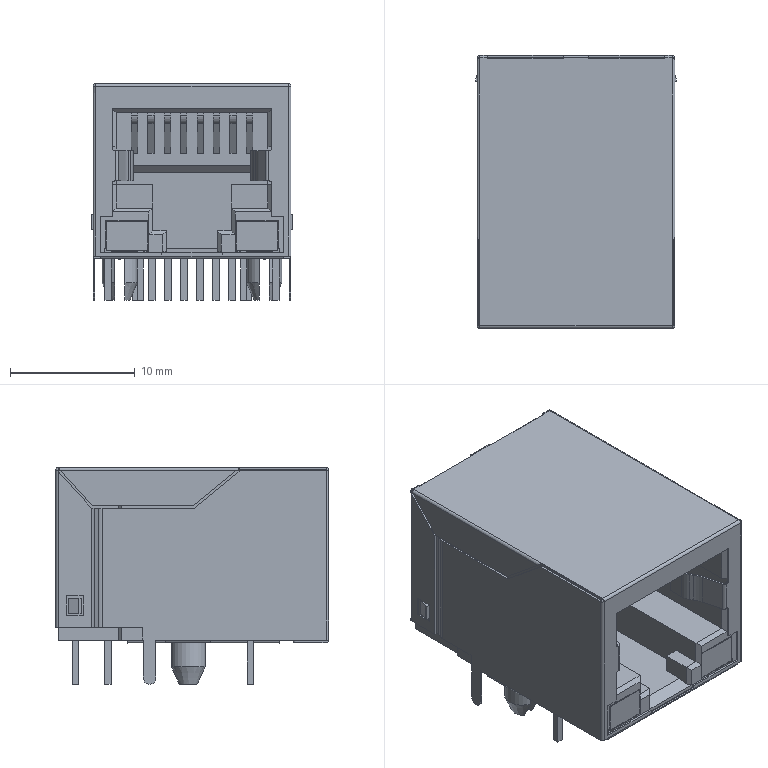Part | NX | features BREP 2 | 2 solids | 622 faces | box 16.054 x 21.854 x 17.342 mm | volume 3367 mm3 | plane 499 | cylinder 86 | spline 29 | sphere 4 | cone 4 | commonest cylinder face diameters 0.405 x19 0.202 x9 0.989 x8 1.393 x8 0.304 x4 1.315 x4